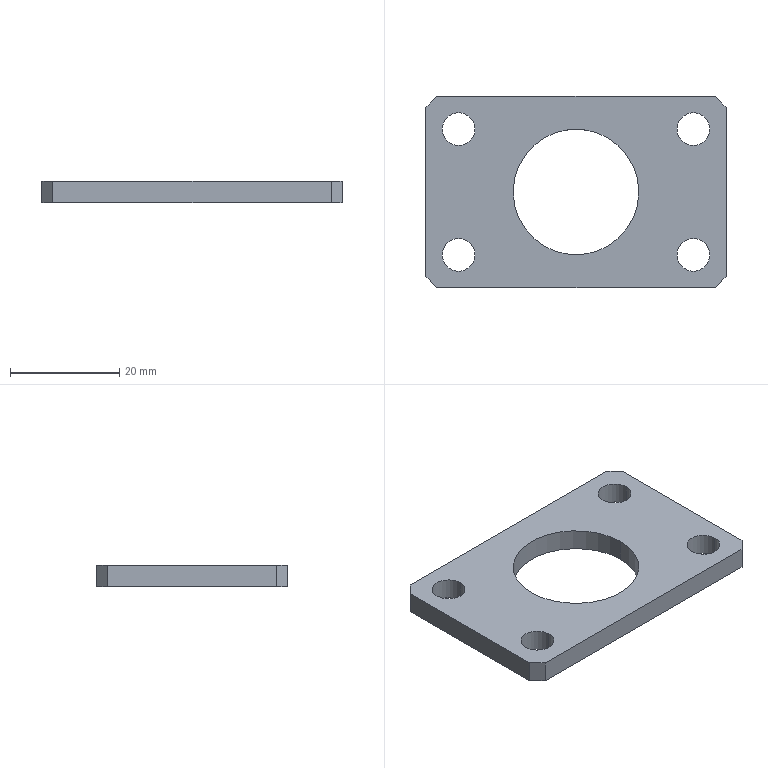Part | SolidWorks | features Chamfer 1, Extrusion 1, ICE 1, MirrorPattern 1 | 1 solid | 20 faces | box 55 x 35 x 4 mm | volume 5554 mm3 | cylinder 10 | plane 10 | commonest cylinder face diameters 6 x8 23 x2
STEP:
#1=CARTESIAN_POINT('',(-18.5,-11.5,-2.));
#2=VERTEX_POINT('',#1);
#3=CARTESIAN_POINT('',(-24.5,-11.5,-2.));
#4=VERTEX_POINT('',#3);
#5=CARTESIAN_POINT('',(-21.5,-11.5,-2.));
#6=DIRECTION('',(0.,0.,-1.));
#7=DIRECTION('',(-1.,0.,0.));
#8=AXIS2_PLACEMENT_3D('',#5,#6,#7);
#9=CIRCLE('',#8,3.);
#10=EDGE_CURVE('',#2,#4,#9,.T.);
#11=ORIENTED_EDGE('',*,*,#10,.T.);
#12=CARTESIAN_POINT('',(-24.5,-11.5,2.));
#13=VERTEX_POINT('',#12);
#14=CARTESIAN_POINT('',(-24.5,-11.5,-2.001));
#15=DIRECTION('',(0.,0.,1.));
#16=VECTOR('',#15,1000.);
#17=LINE('',#14,#16);
#18=EDGE_CURVE('',#4,#13,#17,.T.);
#19=ORIENTED_EDGE('',*,*,#18,.T.);
#20=CARTESIAN_POINT('',(-18.5,-11.5,2.));
#21=VERTEX_POINT('',#20);
#22=CARTESIAN_POINT('',(-21.5,-11.5,2.));
#23=DIRECTION('',(0.,0.,-1.));
#24=DIRECTION('',(1.,0.,0.));
#25=AXIS2_PLACEMENT_3D('',#22,#23,#24);
#26=CIRCLE('',#25,3.);
#27=EDGE_CURVE('',#21,#13,#26,.T.);
#28=ORIENTED_EDGE('',*,*,#27,.F.);
#29=CARTESIAN_POINT('',(-18.5,-11.5,-2.001));
#30=DIRECTION('',(0.,0.,1.));
#31=VECTOR('',#30,1000.);
#32=LINE('',#29,#31);
#33=EDGE_CURVE('',#2,#21,#32,.T.);
#34=ORIENTED_EDGE('',*,*,#33,.F.);
#35=EDGE_LOOP('',(#11,#19,#28,#34));
#36=FACE_OUTER_BOUND('',#35,.T.);
#37=CARTESIAN_POINT('',(-21.5,-11.5,-2.001));
#38=DIRECTION('',(0.,0.,1.));
#39=DIRECTION('',(1.,0.,0.));
#40=AXIS2_PLACEMENT_3D('',#37,#38,#39);
#41=CYLINDRICAL_SURFACE('',#40,3.);
#42=ADVANCED_FACE('',(#36),#41,.F.);
#43=CARTESIAN_POINT('',(24.5,-11.5,-2.));
#44=VERTEX_POINT('',#43);
#45=CARTESIAN_POINT('',(18.5,-11.5,-2.));
#46=VERTEX_POINT('',#45);
#47=CARTESIAN_POINT('',(21.5,-11.5,-2.));
#48=DIRECTION('',(0.,0.,-1.));
#49=DIRECTION('',(-1.,0.,0.));
#50=AXIS2_PLACEMENT_3D('',#47,#48,#49);
#51=CIRCLE('',#50,3.);
#52=EDGE_CURVE('',#44,#46,#51,.T.);
#53=ORIENTED_EDGE('',*,*,#52,.T.);
#54=CARTESIAN_POINT('',(18.5,-11.5,2.));
#55=VERTEX_POINT('',#54);
#56=CARTESIAN_POINT('',(18.5,-11.5,-2.001));
#57=DIRECTION('',(0.,0.,1.));
#58=VECTOR('',#57,1000.);
#59=LINE('',#56,#58);
#60=EDGE_CURVE('',#46,#55,#59,.T.);
#61=ORIENTED_EDGE('',*,*,#60,.T.);
#62=CARTESIAN_POINT('',(24.5,-11.5,2.));
#63=VERTEX_POINT('',#62);
#64=CARTESIAN_POINT('',(21.5,-11.5,2.));
#65=DIRECTION('',(0.,0.,-1.));
#66=DIRECTION('',(1.,0.,0.));
#67=AXIS2_PLACEMENT_3D('',#64,#65,#66);
#68=CIRCLE('',#67,3.);
#69=EDGE_CURVE('',#63,#55,#68,.T.);
#70=ORIENTED_EDGE('',*,*,#69,.F.);
#71=CARTESIAN_POINT('',(24.5,-11.5,-2.001));
#72=DIRECTION('',(0.,0.,1.));
#73=VECTOR('',#72,1000.);
#74=LINE('',#71,#73);
#75=EDGE_CURVE('',#44,#63,#74,.T.);
#76=ORIENTED_EDGE('',*,*,#75,.F.);
#77=EDGE_LOOP('',(#53,#61,#70,#76));
#78=FACE_OUTER_BOUND('',#77,.T.);
#79=CARTESIAN_POINT('',(21.5,-11.5,-2.001));
#80=DIRECTION('',(0.,0.,1.));
#81=DIRECTION('',(1.,0.,0.));
#82=AXIS2_PLACEMENT_3D('',#79,#80,#81);
#83=CYLINDRICAL_SURFACE('',#82,3.);
#84=ADVANCED_FACE('',(#78),#83,.F.);
#85=CARTESIAN_POINT('',(-24.5,11.5,-2.));
#86=VERTEX_POINT('',#85);
#87=CARTESIAN_POINT('',(-18.5,11.5,-2.));
#88=VERTEX_POINT('',#87);
#89=CARTESIAN_POINT('',(-21.5,11.5,-2.));
#90=DIRECTION('',(0.,0.,1.));
#91=DIRECTION('',(-1.,0.,0.));
#92=AXIS2_PLACEMENT_3D('',#89,#90,#91);
#93=CIRCLE('',#92,3.);
#94=EDGE_CURVE('',#86,#88,#93,.T.);
#95=ORIENTED_EDGE('',*,*,#94,.F.);
#96=CARTESIAN_POINT('',(-24.5,11.5,2.));
#97=VERTEX_POINT('',#96);
#98=CARTESIAN_POINT('',(-24.5,11.5,-2.001));
#99=DIRECTION('',(0.,0.,1.));
#100=VECTOR('',#99,1000.);
#101=LINE('',#98,#100);
#102=EDGE_CURVE('',#86,#97,#101,.T.);
#103=ORIENTED_EDGE('',*,*,#102,.T.);
#104=CARTESIAN_POINT('',(-18.5,11.5,2.));
#105=VERTEX_POINT('',#104);
#106=CARTESIAN_POINT('',(-21.5,11.5,2.));
#107=DIRECTION('',(0.,0.,1.));
#108=DIRECTION('',(1.,0.,0.));
#109=AXIS2_PLACEMENT_3D('',#106,#107,#108);
#110=CIRCLE('',#109,3.);
#111=EDGE_CURVE('',#97,#105,#110,.T.);
#112=ORIENTED_EDGE('',*,*,#111,.T.);
#113=CARTESIAN_POINT('',(-18.5,11.5,-2.001));
#114=DIRECTION('',(0.,0.,1.));
#115=VECTOR('',#114,1000.);
#116=LINE('',#113,#115);
#117=EDGE_CURVE('',#88,#105,#116,.T.);
#118=ORIENTED_EDGE('',*,*,#117,.F.);
#119=EDGE_LOOP('',(#95,#103,#112,#118));
#120=FACE_OUTER_BOUND('',#119,.T.);
#121=CARTESIAN_POINT('',(-21.5,11.5,-2.001));
#122=DIRECTION('',(0.,0.,1.));
#123=DIRECTION('',(1.,0.,0.));
#124=AXIS2_PLACEMENT_3D('',#121,#122,#123);
#125=CYLINDRICAL_SURFACE('',#124,3.);
#126=ADVANCED_FACE('',(#120),#125,.F.);
#127=CARTESIAN_POINT('',(18.5,11.5,-2.));
#128=VERTEX_POINT('',#127);
#129=CARTESIAN_POINT('',(24.5,11.5,-2.));
#130=VERTEX_POINT('',#129);
#131=CARTESIAN_POINT('',(21.5,11.5,-2.));
#132=DIRECTION('',(0.,0.,1.));
#133=DIRECTION('',(-1.,0.,0.));
#134=AXIS2_PLACEMENT_3D('',#131,#132,#133);
#135=CIRCLE('',#134,3.);
#136=EDGE_CURVE('',#128,#130,#135,.T.);
#137=ORIENTED_EDGE('',*,*,#136,.F.);
#138=CARTESIAN_POINT('',(18.5,11.5,2.));
#139=VERTEX_POINT('',#138);
#140=CARTESIAN_POINT('',(18.5,11.5,-2.001));
#141=DIRECTION('',(0.,0.,1.));
#142=VECTOR('',#141,1000.);
#143=LINE('',#140,#142);
#144=EDGE_CURVE('',#128,#139,#143,.T.);
#145=ORIENTED_EDGE('',*,*,#144,.T.);
#146=CARTESIAN_POINT('',(24.5,11.5,2.));
#147=VERTEX_POINT('',#146);
#148=CARTESIAN_POINT('',(21.5,11.5,2.));
#149=DIRECTION('',(0.,0.,1.));
#150=DIRECTION('',(1.,0.,0.));
#151=AXIS2_PLACEMENT_3D('',#148,#149,#150);
#152=CIRCLE('',#151,3.);
#153=EDGE_CURVE('',#139,#147,#152,.T.);
#154=ORIENTED_EDGE('',*,*,#153,.T.);
#155=CARTESIAN_POINT('',(24.5,11.5,-2.001));
#156=DIRECTION('',(0.,0.,1.));
#157=VECTOR('',#156,1000.);
#158=LINE('',#155,#157);
#159=EDGE_CURVE('',#130,#147,#158,.T.);
#160=ORIENTED_EDGE('',*,*,#159,.F.);
#161=EDGE_LOOP('',(#137,#145,#154,#160));
#162=FACE_OUTER_BOUND('',#161,.T.);
#163=CARTESIAN_POINT('',(21.5,11.5,-2.001));
#164=DIRECTION('',(0.,0.,1.));
#165=DIRECTION('',(1.,0.,0.));
#166=AXIS2_PLACEMENT_3D('',#163,#164,#165);
#167=CYLINDRICAL_SURFACE('',#166,3.);
#168=ADVANCED_FACE('',(#162),#167,.F.);
#169=CARTESIAN_POINT('',(-11.5,0.,2.));
#170=VERTEX_POINT('',#169);
#171=CARTESIAN_POINT('',(11.5,0.,2.));
#172=VERTEX_POINT('',#171);
#173=CARTESIAN_POINT('',(0.,0.,2.));
#174=DIRECTION('',(0.,0.,1.));
#175=DIRECTION('',(1.,0.,0.));
#176=AXIS2_PLACEMENT_3D('',#173,#174,#175);
#177=CIRCLE('',#176,11.5);
#178=EDGE_CURVE('',#170,#172,#177,.T.);
#179=ORIENTED_EDGE('',*,*,#178,.T.);
#180=CARTESIAN_POINT('',(11.5,0.,-2.));
#181=VERTEX_POINT('',#180);
#182=CARTESIAN_POINT('',(11.5,0.,2.));
#183=DIRECTION('',(0.,0.,-1.));
#184=VECTOR('',#183,1000.);
#185=LINE('',#182,#184);
#186=EDGE_CURVE('',#172,#181,#185,.T.);
#187=ORIENTED_EDGE('',*,*,#186,.T.);
#188=CARTESIAN_POINT('',(-11.5,0.,-2.));
#189=VERTEX_POINT('',#188);
#190=CARTESIAN_POINT('',(0.,0.,-2.));
#191=DIRECTION('',(0.,0.,1.));
#192=DIRECTION('',(1.,0.,0.));
#193=AXIS2_PLACEMENT_3D('',#190,#191,#192);
#194=CIRCLE('',#193,11.5);
#195=EDGE_CURVE('',#189,#181,#194,.T.);
#196=ORIENTED_EDGE('',*,*,#195,.F.);
#197=CARTESIAN_POINT('',(-11.5,0.,2.));
#198=DIRECTION('',(0.,0.,-1.));
#199=VECTOR('',#198,1000.);
#200=LINE('',#197,#199);
#201=EDGE_CURVE('',#170,#189,#200,.T.);
#202=ORIENTED_EDGE('',*,*,#201,.F.);
#203=EDGE_LOOP('',(#179,#187,#196,#202));
#204=FACE_OUTER_BOUND('',#203,.T.);
#205=CARTESIAN_POINT('',(0.,0.,2.));
#206=DIRECTION('',(0.,0.,-1.));
#207=DIRECTION('',(-1.,0.,0.));
#208=AXIS2_PLACEMENT_3D('',#205,#206,#207);
#209=CYLINDRICAL_SURFACE('',#208,11.5);
#210=ADVANCED_FACE('',(#204),#209,.F.);
#211=ORIENTED_EDGE('',*,*,#27,.T.);
#212=CARTESIAN_POINT('',(-21.5,-11.5,2.));
#213=DIRECTION('',(0.,0.,-1.));
#214=DIRECTION('',(1.,0.,0.));
#215=AXIS2_PLACEMENT_3D('',#212,#213,#214);
#216=CIRCLE('',#215,3.);
#217=EDGE_CURVE('',#13,#21,#216,.T.);
#218=ORIENTED_EDGE('',*,*,#217,.T.);
#219=EDGE_LOOP('',(#211,#218));
#220=FACE_BOUND('',#219,.T.);
#221=ORIENTED_EDGE('',*,*,#69,.T.);
#222=CARTESIAN_POINT('',(21.5,-11.5,2.));
#223=DIRECTION('',(0.,0.,-1.));
#224=DIRECTION('',(1.,0.,0.));
#225=AXIS2_PLACEMENT_3D('',#222,#223,#224);
#226=CIRCLE('',#225,3.);
#227=EDGE_CURVE('',#55,#63,#226,.T.);
#228=ORIENTED_EDGE('',*,*,#227,.T.);
#229=EDGE_LOOP('',(#221,#228));
#230=FACE_BOUND('',#229,.T.);
#231=CARTESIAN_POINT('',(-21.5,11.5,2.));
#232=DIRECTION('',(0.,0.,1.));
#233=DIRECTION('',(1.,0.,0.));
#234=AXIS2_PLACEMENT_3D('',#231,#232,#233);
#235=CIRCLE('',#234,3.);
#236=EDGE_CURVE('',#105,#97,#235,.T.);
#237=ORIENTED_EDGE('',*,*,#236,.F.);
#238=ORIENTED_EDGE('',*,*,#111,.F.);
#239=EDGE_LOOP('',(#237,#238));
#240=FACE_BOUND('',#239,.T.);
#241=CARTESIAN_POINT('',(21.5,11.5,2.));
#242=DIRECTION('',(0.,0.,1.));
#243=DIRECTION('',(1.,0.,0.));
#244=AXIS2_PLACEMENT_3D('',#241,#242,#243);
#245=CIRCLE('',#244,3.);
#246=EDGE_CURVE('',#147,#139,#245,.T.);
#247=ORIENTED_EDGE('',*,*,#246,.F.);
#248=ORIENTED_EDGE('',*,*,#153,.F.);
#249=EDGE_LOOP('',(#247,#248));
#250=FACE_BOUND('',#249,.T.);
#251=CARTESIAN_POINT('',(27.5,-15.5,2.));
#252=VERTEX_POINT('',#251);
#253=CARTESIAN_POINT('',(27.5,15.5,2.));
#254=VERTEX_POINT('',#253);
#255=CARTESIAN_POINT('',(27.5,-17.5,2.));
#256=DIRECTION('',(0.,1.,0.));
#257=VECTOR('',#256,1000.);
#258=LINE('',#255,#257);
#259=EDGE_CURVE('',#252,#254,#258,.T.);
#260=ORIENTED_EDGE('',*,*,#259,.T.);
#261=CARTESIAN_POINT('',(25.5,17.5,2.));
#262=VERTEX_POINT('',#261);
#263=CARTESIAN_POINT('',(25.5,17.5,2.));
#264=DIRECTION('',(-0.7071,0.7071,0.));
#265=VECTOR('',#264,1000.);
#266=LINE('',#263,#265);
#267=EDGE_CURVE('',#254,#262,#266,.T.);
#268=ORIENTED_EDGE('',*,*,#267,.T.);
#269=CARTESIAN_POINT('',(-25.5,17.5,2.));
#270=VERTEX_POINT('',#269);
#271=CARTESIAN_POINT('',(-27.5,17.5,2.));
#272=DIRECTION('',(-1.,0.,0.));
#273=VECTOR('',#272,1000.);
#274=LINE('',#271,#273);
#275=EDGE_CURVE('',#262,#270,#274,.T.);
#276=ORIENTED_EDGE('',*,*,#275,.T.);
#277=CARTESIAN_POINT('',(-27.5,15.5,2.));
#278=VERTEX_POINT('',#277);
#279=CARTESIAN_POINT('',(-27.5,15.5,2.));
#280=DIRECTION('',(-0.7071,-0.7071,0.));
#281=VECTOR('',#280,1000.);
#282=LINE('',#279,#281);
#283=EDGE_CURVE('',#270,#278,#282,.T.);
#284=ORIENTED_EDGE('',*,*,#283,.T.);
#285=CARTESIAN_POINT('',(-27.5,-15.5,2.));
#286=VERTEX_POINT('',#285);
#287=CARTESIAN_POINT('',(-27.5,-17.5,2.));
#288=DIRECTION('',(0.,-1.,0.));
#289=VECTOR('',#288,1000.);
#290=LINE('',#287,#289);
#291=EDGE_CURVE('',#278,#286,#290,.T.);
#292=ORIENTED_EDGE('',*,*,#291,.T.);
#293=CARTESIAN_POINT('',(-25.5,-17.5,2.));
#294=VERTEX_POINT('',#293);
#295=CARTESIAN_POINT('',(-25.5,-17.5,2.));
#296=DIRECTION('',(0.7071,-0.7071,0.));
#297=VECTOR('',#296,1000.);
#298=LINE('',#295,#297);
#299=EDGE_CURVE('',#286,#294,#298,.T.);
#300=ORIENTED_EDGE('',*,*,#299,.T.);
#301=CARTESIAN_POINT('',(25.5,-17.5,2.));
#302=VERTEX_POINT('',#301);
#303=CARTESIAN_POINT('',(-27.5,-17.5,2.));
#304=DIRECTION('',(1.,0.,0.));
#305=VECTOR('',#304,1000.);
#306=LINE('',#303,#305);
#307=EDGE_CURVE('',#294,#302,#306,.T.);
#308=ORIENTED_EDGE('',*,*,#307,.T.);
#309=CARTESIAN_POINT('',(27.5,-15.5,2.));
#310=DIRECTION('',(0.7071,0.7071,0.));
#311=VECTOR('',#310,1000.);
#312=LINE('',#309,#311);
#313=EDGE_CURVE('',#302,#252,#312,.T.);
#314=ORIENTED_EDGE('',*,*,#313,.T.);
#315=EDGE_LOOP('',(#260,#268,#276,#284,#292,#300,#308,#314));
#316=FACE_OUTER_BOUND('',#315,.T.);
#317=ORIENTED_EDGE('',*,*,#178,.F.);
#318=CARTESIAN_POINT('',(0.,0.,2.));
#319=DIRECTION('',(0.,0.,1.));
#320=DIRECTION('',(1.,0.,0.));
#321=AXIS2_PLACEMENT_3D('',#318,#319,#320);
#322=CIRCLE('',#321,11.5);
#323=EDGE_CURVE('',#172,#170,#322,.T.);
#324=ORIENTED_EDGE('',*,*,#323,.F.);
#325=EDGE_LOOP('',(#317,#324));
#326=FACE_BOUND('',#325,.T.);
#327=CARTESIAN_POINT('',(0.,0.,2.));
#328=DIRECTION('',(0.,0.,-1.));
#329=DIRECTION('',(-1.,0.,0.));
#330=AXIS2_PLACEMENT_3D('',#327,#328,#329);
#331=PLANE('',#330);
#332=ADVANCED_FACE('',(#220,#230,#240,#250,#316,#326),#331,.F.);
#333=ORIENTED_EDGE('',*,*,#10,.F.);
#334=CARTESIAN_POINT('',(-21.5,-11.5,-2.));
#335=DIRECTION('',(0.,0.,-1.));
#336=DIRECTION('',(-1.,0.,0.));
#337=AXIS2_PLACEMENT_3D('',#334,#335,#336);
#338=CIRCLE('',#337,3.);
#339=EDGE_CURVE('',#4,#2,#338,.T.);
#340=ORIENTED_EDGE('',*,*,#339,.F.);
#341=EDGE_LOOP('',(#333,#340));
#342=FACE_BOUND('',#341,.T.);
#343=ORIENTED_EDGE('',*,*,#52,.F.);
#344=CARTESIAN_POINT('',(21.5,-11.5,-2.));
#345=DIRECTION('',(0.,0.,-1.));
#346=DIRECTION('',(-1.,0.,0.));
#347=AXIS2_PLACEMENT_3D('',#344,#345,#346);
#348=CIRCLE('',#347,3.);
#349=EDGE_CURVE('',#46,#44,#348,.T.);
#350=ORIENTED_EDGE('',*,*,#349,.F.);
#351=EDGE_LOOP('',(#343,#350));
#352=FACE_BOUND('',#351,.T.);
#353=CARTESIAN_POINT('',(-21.5,11.5,-2.));
#354=DIRECTION('',(0.,0.,1.));
#355=DIRECTION('',(-1.,0.,0.));
#356=AXIS2_PLACEMENT_3D('',#353,#354,#355);
#357=CIRCLE('',#356,3.);
#358=EDGE_CURVE('',#88,#86,#357,.T.);
#359=ORIENTED_EDGE('',*,*,#358,.T.);
#360=ORIENTED_EDGE('',*,*,#94,.T.);
#361=EDGE_LOOP('',(#359,#360));
#362=FACE_BOUND('',#361,.T.);
#363=CARTESIAN_POINT('',(21.5,11.5,-2.));
#364=DIRECTION('',(0.,0.,1.));
#365=DIRECTION('',(-1.,0.,0.));
#366=AXIS2_PLACEMENT_3D('',#363,#364,#365);
#367=CIRCLE('',#366,3.);
#368=EDGE_CURVE('',#130,#128,#367,.T.);
#369=ORIENTED_EDGE('',*,*,#368,.T.);
#370=ORIENTED_EDGE('',*,*,#136,.T.);
#371=EDGE_LOOP('',(#369,#370));
#372=FACE_BOUND('',#371,.T.);
#373=CARTESIAN_POINT('',(25.5,17.5,-2.));
#374=VERTEX_POINT('',#373);
#375=CARTESIAN_POINT('',(-25.5,17.5,-2.));
#376=VERTEX_POINT('',#375);
#377=CARTESIAN_POINT('',(-27.5,17.5,-2.));
#378=DIRECTION('',(-1.,0.,0.));
#379=VECTOR('',#378,1000.);
#380=LINE('',#377,#379);
#381=EDGE_CURVE('',#374,#376,#380,.T.);
#382=ORIENTED_EDGE('',*,*,#381,.F.);
#383=CARTESIAN_POINT('',(27.5,15.5,-2.));
#384=VERTEX_POINT('',#383);
#385=CARTESIAN_POINT('',(21.5,21.5,-2.));
#386=DIRECTION('',(0.7071,-0.7071,0.));
#387=VECTOR('',#386,1000.);
#388=LINE('',#385,#387);
#389=EDGE_CURVE('',#374,#384,#388,.T.);
#390=ORIENTED_EDGE('',*,*,#389,.T.);
#391=CARTESIAN_POINT('',(27.5,-15.5,-2.));
#392=VERTEX_POINT('',#391);
#393=CARTESIAN_POINT('',(27.5,-17.5,-2.));
#394=DIRECTION('',(0.,1.,0.));
#395=VECTOR('',#394,1000.);
#396=LINE('',#393,#395);
#397=EDGE_CURVE('',#392,#384,#396,.T.);
#398=ORIENTED_EDGE('',*,*,#397,.F.);
#399=CARTESIAN_POINT('',(25.5,-17.5,-2.));
#400=VERTEX_POINT('',#399);
#401=CARTESIAN_POINT('',(21.5,-21.5,-2.));
#402=DIRECTION('',(-0.7071,-0.7071,0.));
#403=VECTOR('',#402,1000.);
#404=LINE('',#401,#403);
#405=EDGE_CURVE('',#392,#400,#404,.T.);
#406=ORIENTED_EDGE('',*,*,#405,.T.);
#407=CARTESIAN_POINT('',(-25.5,-17.5,-2.));
#408=VERTEX_POINT('',#407);
#409=CARTESIAN_POINT('',(-27.5,-17.5,-2.));
#410=DIRECTION('',(1.,0.,0.));
#411=VECTOR('',#410,1000.);
#412=LINE('',#409,#411);
#413=EDGE_CURVE('',#408,#400,#412,.T.);
#414=ORIENTED_EDGE('',*,*,#413,.F.);
#415=CARTESIAN_POINT('',(-27.5,-15.5,-2.));
#416=VERTEX_POINT('',#415);
#417=CARTESIAN_POINT('',(-21.5,-21.5,-2.));
#418=DIRECTION('',(-0.7071,0.7071,0.));
#419=VECTOR('',#418,1000.);
#420=LINE('',#417,#419);
#421=EDGE_CURVE('',#408,#416,#420,.T.);
#422=ORIENTED_EDGE('',*,*,#421,.T.);
#423=CARTESIAN_POINT('',(-27.5,15.5,-2.));
#424=VERTEX_POINT('',#423);
#425=CARTESIAN_POINT('',(-27.5,-17.5,-2.));
#426=DIRECTION('',(0.,-1.,0.));
#427=VECTOR('',#426,1000.);
#428=LINE('',#425,#427);
#429=EDGE_CURVE('',#424,#416,#428,.T.);
#430=ORIENTED_EDGE('',*,*,#429,.F.);
#431=CARTESIAN_POINT('',(-21.5,21.5,-2.));
#432=DIRECTION('',(0.7071,0.7071,0.));
#433=VECTOR('',#432,1000.);
#434=LINE('',#431,#433);
#435=EDGE_CURVE('',#424,#376,#434,.T.);
#436=ORIENTED_EDGE('',*,*,#435,.T.);
#437=EDGE_LOOP('',(#382,#390,#398,#406,#414,#422,#430,#436));
#438=FACE_OUTER_BOUND('',#437,.T.);
#439=ORIENTED_EDGE('',*,*,#195,.T.);
#440=CARTESIAN_POINT('',(0.,0.,-2.));
#441=DIRECTION('',(0.,0.,1.));
#442=DIRECTION('',(1.,0.,0.));
#443=AXIS2_PLACEMENT_3D('',#440,#441,#442);
#444=CIRCLE('',#443,11.5);
#445=EDGE_CURVE('',#181,#189,#444,.T.);
#446=ORIENTED_EDGE('',*,*,#445,.T.);
#447=EDGE_LOOP('',(#439,#446));
#448=FACE_BOUND('',#447,.T.);
#449=CARTESIAN_POINT('',(0.,0.,-2.));
#450=DIRECTION('',(0.,0.,-1.));
#451=DIRECTION('',(-1.,0.,0.));
#452=AXIS2_PLACEMENT_3D('',#449,#450,#451);
#453=PLANE('',#452);
#454=ADVANCED_FACE('',(#342,#352,#362,#372,#438,#448),#453,.T.);
#455=ORIENTED_EDGE('',*,*,#397,.T.);
#456=CARTESIAN_POINT('',(27.5,15.5,2.));
#457=DIRECTION('',(0.,0.,1.));
#458=VECTOR('',#457,1000.);
#459=LINE('',#456,#458);
#460=EDGE_CURVE('',#384,#254,#459,.T.);
#461=ORIENTED_EDGE('',*,*,#460,.T.);
#462=ORIENTED_EDGE('',*,*,#259,.F.);
#463=CARTESIAN_POINT('',(27.5,-15.5,2.));
#464=DIRECTION('',(0.,0.,-1.));
#465=VECTOR('',#464,1000.);
#466=LINE('',#463,#465);
#467=EDGE_CURVE('',#252,#392,#466,.T.);
#468=ORIENTED_EDGE('',*,*,#467,.T.);
#469=EDGE_LOOP('',(#455,#461,#462,#468));
#470=FACE_OUTER_BOUND('',#469,.T.);
#471=CARTESIAN_POINT('',(27.5,-17.5,2.));
#472=DIRECTION('',(-1.,0.,0.));
#473=DIRECTION('',(0.,0.,1.));
#474=AXIS2_PLACEMENT_3D('',#471,#472,#473);
#475=PLANE('',#474);
#476=ADVANCED_FACE('',(#470),#475,.F.);
#477=ORIENTED_EDGE('',*,*,#275,.F.);
#478=CARTESIAN_POINT('',(25.5,17.5,2.));
#479=DIRECTION('',(0.,0.,-1.));
#480=VECTOR('',#479,1000.);
#481=LINE('',#478,#480);
#482=EDGE_CURVE('',#262,#374,#481,.T.);
#483=ORIENTED_EDGE('',*,*,#482,.T.);
#484=ORIENTED_EDGE('',*,*,#381,.T.);
#485=CARTESIAN_POINT('',(-25.5,17.5,2.));
#486=DIRECTION('',(0.,0.,1.));
#487=VECTOR('',#486,1000.);
#488=LINE('',#485,#487);
#489=EDGE_CURVE('',#376,#270,#488,.T.);
#490=ORIENTED_EDGE('',*,*,#489,.T.);
#491=EDGE_LOOP('',(#477,#483,#484,#490));
#492=FACE_OUTER_BOUND('',#491,.T.);
#493=CARTESIAN_POINT('',(-27.5,17.5,2.));
#494=DIRECTION('',(0.,-1.,0.));
#495=DIRECTION('',(0.,0.,-1.));
#496=AXIS2_PLACEMENT_3D('',#493,#494,#495);
#497=PLANE('',#496);
#498=ADVANCED_FACE('',(#492),#497,.F.);
#499=ORIENTED_EDGE('',*,*,#291,.F.);
#500=CARTESIAN_POINT('',(-27.5,15.5,2.));
#501=DIRECTION('',(0.,0.,-1.));
#502=VECTOR('',#501,1000.);
#503=LINE('',#500,#502);
#504=EDGE_CURVE('',#278,#424,#503,.T.);
#505=ORIENTED_EDGE('',*,*,#504,.T.);
#506=ORIENTED_EDGE('',*,*,#429,.T.);
#507=CARTESIAN_POINT('',(-27.5,-15.5,2.));
#508=DIRECTION('',(0.,0.,1.));
#509=VECTOR('',#508,1000.);
#510=LINE('',#507,#509);
#511=EDGE_CURVE('',#416,#286,#510,.T.);
#512=ORIENTED_EDGE('',*,*,#511,.T.);
#513=EDGE_LOOP('',(#499,#505,#506,#512));
#514=FACE_OUTER_BOUND('',#513,.T.);
#515=CARTESIAN_POINT('',(-27.5,-17.5,2.));
#516=DIRECTION('',(1.,0.,0.));
#517=DIRECTION('',(0.,0.,-1.));
#518=AXIS2_PLACEMENT_3D('',#515,#516,#517);
#519=PLANE('',#518);
#520=ADVANCED_FACE('',(#514),#519,.F.);
#521=ORIENTED_EDGE('',*,*,#413,.T.);
#522=CARTESIAN_POINT('',(25.5,-17.5,2.));
#523=DIRECTION('',(0.,0.,1.));
#524=VECTOR('',#523,1000.);
#525=LINE('',#522,#524);
#526=EDGE_CURVE('',#400,#302,#525,.T.);
#527=ORIENTED_EDGE('',*,*,#526,.T.);
#528=ORIENTED_EDGE('',*,*,#307,.F.);
#529=CARTESIAN_POINT('',(-25.5,-17.5,2.));
#530=DIRECTION('',(0.,0.,-1.));
#531=VECTOR('',#530,1000.);
#532=LINE('',#529,#531);
#533=EDGE_CURVE('',#294,#408,#532,.T.);
#534=ORIENTED_EDGE('',*,*,#533,.T.);
#535=EDGE_LOOP('',(#521,#527,#528,#534));
#536=FACE_OUTER_BOUND('',#535,.T.);
#537=CARTESIAN_POINT('',(-27.5,-17.5,2.));
#538=DIRECTION('',(0.,1.,0.));
#539=DIRECTION('',(0.,0.,1.));
#540=AXIS2_PLACEMENT_3D('',#537,#538,#539);
#541=PLANE('',#540);
#542=ADVANCED_FACE('',(#536),#541,.F.);
#543=ORIENTED_EDGE('',*,*,#186,.F.);
#544=ORIENTED_EDGE('',*,*,#323,.T.);
#545=ORIENTED_EDGE('',*,*,#201,.T.);
#546=ORIENTED_EDGE('',*,*,#445,.F.);
#547=EDGE_LOOP('',(#543,#544,#545,#546));
#548=FACE_OUTER_BOUND('',#547,.T.);
#549=CARTESIAN_POINT('',(0.,0.,2.));
#550=DIRECTION('',(0.,0.,-1.));
#551=DIRECTION('',(-1.,0.,0.));
#552=AXIS2_PLACEMENT_3D('',#549,#550,#551);
#553=CYLINDRICAL_SURFACE('',#552,11.5);
#554=ADVANCED_FACE('',(#548),#553,.F.);
#555=ORIENTED_EDGE('',*,*,#144,.F.);
#556=ORIENTED_EDGE('',*,*,#368,.F.);
#557=ORIENTED_EDGE('',*,*,#159,.T.);
#558=ORIENTED_EDGE('',*,*,#246,.T.);
#559=EDGE_LOOP('',(#555,#556,#557,#558));
#560=FACE_OUTER_BOUND('',#559,.T.);
#561=CARTESIAN_POINT('',(21.5,11.5,-2.001));
#562=DIRECTION('',(0.,0.,1.));
#563=DIRECTION('',(1.,0.,0.));
#564=AXIS2_PLACEMENT_3D('',#561,#562,#563);
#565=CYLINDRICAL_SURFACE('',#564,3.);
#566=ADVANCED_FACE('',(#560),#565,.F.);
#567=ORIENTED_EDGE('',*,*,#102,.F.);
#568=ORIENTED_EDGE('',*,*,#358,.F.);
#569=ORIENTED_EDGE('',*,*,#117,.T.);
#570=ORIENTED_EDGE('',*,*,#236,.T.);
#571=EDGE_LOOP('',(#567,#568,#569,#570));
#572=FACE_OUTER_BOUND('',#571,.T.);
#573=CARTESIAN_POINT('',(-21.5,11.5,-2.001));
#574=DIRECTION('',(0.,0.,1.));
#575=DIRECTION('',(1.,0.,0.));
#576=AXIS2_PLACEMENT_3D('',#573,#574,#575);
#577=CYLINDRICAL_SURFACE('',#576,3.);
#578=ADVANCED_FACE('',(#572),#577,.F.);
#579=ORIENTED_EDGE('',*,*,#267,.F.);
#580=ORIENTED_EDGE('',*,*,#460,.F.);
#581=ORIENTED_EDGE('',*,*,#389,.F.);
#582=ORIENTED_EDGE('',*,*,#482,.F.);
#583=EDGE_LOOP('',(#579,#580,#581,#582));
#584=FACE_OUTER_BOUND('',#583,.T.);
#585=CARTESIAN_POINT('',(25.5,17.5,2.));
#586=DIRECTION('',(-0.7071,-0.7071,0.));
#587=DIRECTION('',(0.,0.,-1.));
#588=AXIS2_PLACEMENT_3D('',#585,#586,#587);
#589=PLANE('',#588);
#590=ADVANCED_FACE('',(#584),#589,.F.);
#591=ORIENTED_EDGE('',*,*,#283,.F.);
#592=ORIENTED_EDGE('',*,*,#489,.F.);
#593=ORIENTED_EDGE('',*,*,#435,.F.);
#594=ORIENTED_EDGE('',*,*,#504,.F.);
#595=EDGE_LOOP('',(#591,#592,#593,#594));
#596=FACE_OUTER_BOUND('',#595,.T.);
#597=CARTESIAN_POINT('',(-27.5,15.5,2.));
#598=DIRECTION('',(0.7071,-0.7071,0.));
#599=DIRECTION('',(0.,0.,-1.));
#600=AXIS2_PLACEMENT_3D('',#597,#598,#599);
#601=PLANE('',#600);
#602=ADVANCED_FACE('',(#596),#601,.F.);
#603=ORIENTED_EDGE('',*,*,#313,.F.);
#604=ORIENTED_EDGE('',*,*,#526,.F.);
#605=ORIENTED_EDGE('',*,*,#405,.F.);
#606=ORIENTED_EDGE('',*,*,#467,.F.);
#607=EDGE_LOOP('',(#603,#604,#605,#606));
#608=FACE_OUTER_BOUND('',#607,.T.);
#609=CARTESIAN_POINT('',(27.5,-15.5,2.));
#610=DIRECTION('',(-0.7071,0.7071,0.));
#611=DIRECTION('',(0.,0.,-1.));
#612=AXIS2_PLACEMENT_3D('',#609,#610,#611);
#613=PLANE('',#612);
#614=ADVANCED_FACE('',(#608),#613,.F.);
#615=ORIENTED_EDGE('',*,*,#299,.F.);
#616=ORIENTED_EDGE('',*,*,#511,.F.);
#617=ORIENTED_EDGE('',*,*,#421,.F.);
#618=ORIENTED_EDGE('',*,*,#533,.F.);
#619=EDGE_LOOP('',(#615,#616,#617,#618));
#620=FACE_OUTER_BOUND('',#619,.T.);
#621=CARTESIAN_POINT('',(-25.5,-17.5,2.));
#622=DIRECTION('',(0.7071,0.7071,0.));
#623=DIRECTION('',(0.,0.,-1.));
#624=AXIS2_PLACEMENT_3D('',#621,#622,#623);
#625=PLANE('',#624);
#626=ADVANCED_FACE('',(#620),#625,.F.);
#627=ORIENTED_EDGE('',*,*,#60,.F.);
#628=ORIENTED_EDGE('',*,*,#349,.T.);
#629=ORIENTED_EDGE('',*,*,#75,.T.);
#630=ORIENTED_EDGE('',*,*,#227,.F.);
#631=EDGE_LOOP('',(#627,#628,#629,#630));
#632=FACE_OUTER_BOUND('',#631,.T.);
#633=CARTESIAN_POINT('',(21.5,-11.5,-2.001));
#634=DIRECTION('',(0.,0.,1.));
#635=DIRECTION('',(1.,0.,0.));
#636=AXIS2_PLACEMENT_3D('',#633,#634,#635);
#637=CYLINDRICAL_SURFACE('',#636,3.);
#638=ADVANCED_FACE('',(#632),#637,.F.);
#639=ORIENTED_EDGE('',*,*,#18,.F.);
#640=ORIENTED_EDGE('',*,*,#339,.T.);
#641=ORIENTED_EDGE('',*,*,#33,.T.);
#642=ORIENTED_EDGE('',*,*,#217,.F.);
#643=EDGE_LOOP('',(#639,#640,#641,#642));
#644=FACE_OUTER_BOUND('',#643,.T.);
#645=CARTESIAN_POINT('',(-21.5,-11.5,-2.001));
#646=DIRECTION('',(0.,0.,1.));
#647=DIRECTION('',(1.,0.,0.));
#648=AXIS2_PLACEMENT_3D('',#645,#646,#647);
#649=CYLINDRICAL_SURFACE('',#648,3.);
#650=ADVANCED_FACE('',(#644),#649,.F.);
#651=CLOSED_SHELL('',(#42,#84,#126,#168,#210,#332,#454,#476,#498,#520,#542,#554,#566,#578,#590,#602,#614,#626,#638,#650));
#652=MANIFOLD_SOLID_BREP('',#651);
#653=CARTESIAN_POINT('',(0.,0.,0.));
#654=DIRECTION('',(0.,0.,1.));
#655=DIRECTION('',(1.,0.,0.));
#656=AXIS2_PLACEMENT_3D('',#653,#654,#655);
#657=(LENGTH_UNIT()NAMED_UNIT(*)SI_UNIT(.MILLI.,.METRE.));
#658=UNCERTAINTY_MEASURE_WITH_UNIT(LENGTH_MEASURE(0.00001),#657,'','');
#659=(NAMED_UNIT(*)PLANE_ANGLE_UNIT()SI_UNIT($,.RADIAN.));
#660=(NAMED_UNIT(*)SI_UNIT($,.STERADIAN.)SOLID_ANGLE_UNIT());
#661=(GEOMETRIC_REPRESENTATION_CONTEXT(3)GLOBAL_UNCERTAINTY_ASSIGNED_CONTEXT((#658))GLOBAL_UNIT_ASSIGNED_CONTEXT((#657,#659,#660))REPRESENTATION_CONTEXT('',''));
#662=ADVANCED_BREP_SHAPE_REPRESENTATION('',(#652,#656),#661);